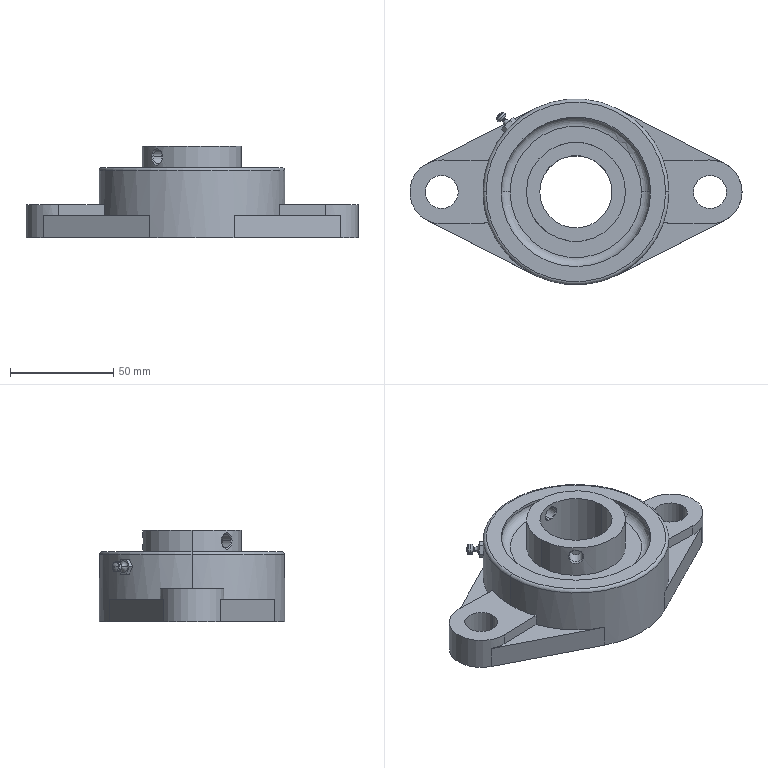Part | STEP file | HDH35_HDH35 | 1 solid | 83 faces | box 161 x 90 x 44.4 mm | volume 197699 mm3 | plane 28 | cylinder 27 | torus 16 | cone 10 | other 2 | commonest cylinder face diameters 6.647 x4 16 x4 48 x4 72.5 x4 31 x3 2 x2